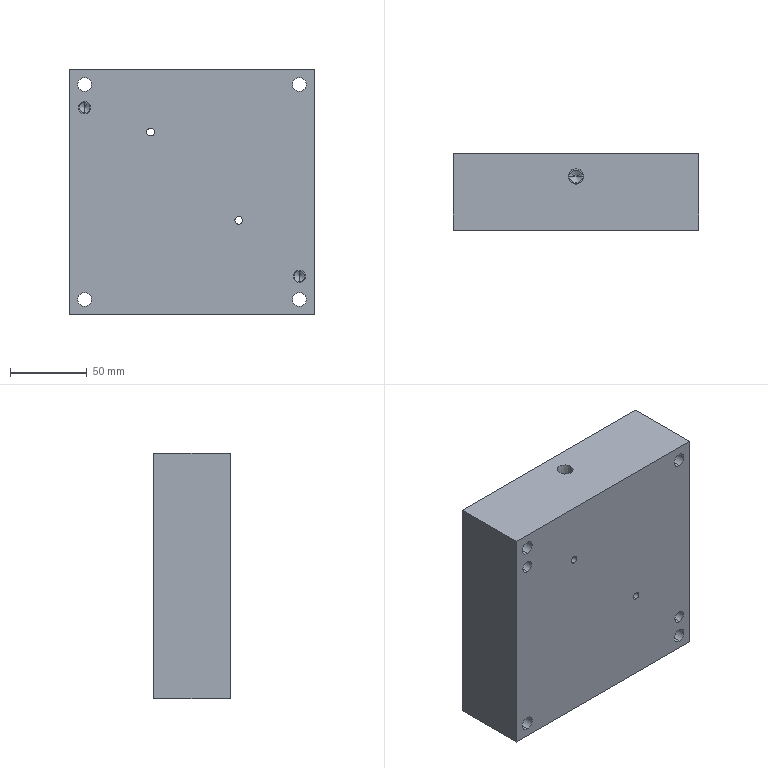Part | STEP file | OP10-111_base block (lower)-L  | 1 solid | 87 faces | box 160 x 50 x 160 mm | volume 1248387 mm3 | cylinder 52 | plane 27 | cone 8 | commonest cylinder face diameters 6 x10 9 x8 14 x8 5 x4 7 x4 8 x4